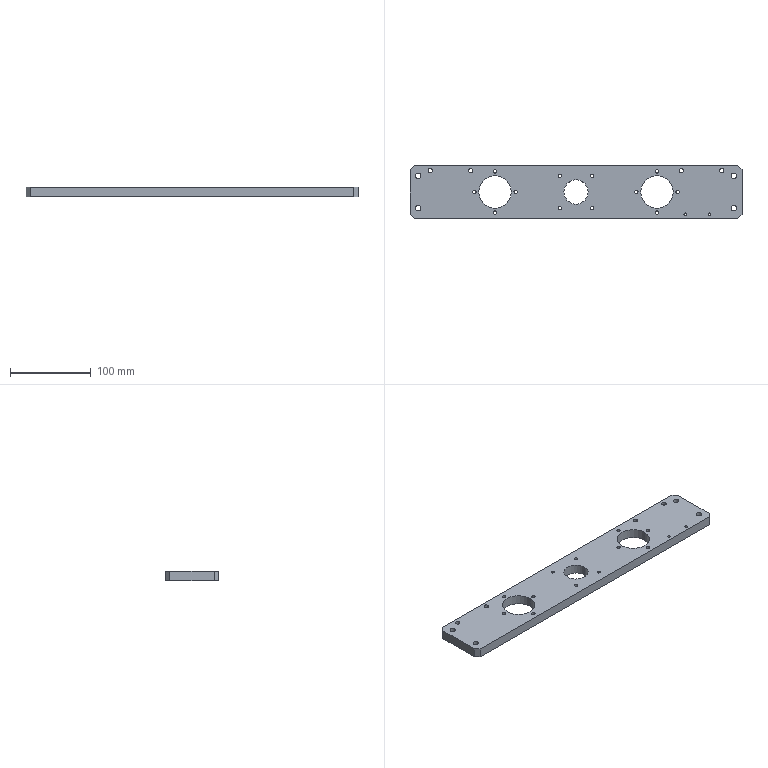Part | SolidWorks | features BaseBody 1 | 1 solid | 60 faces | box 410 x 65 x 12 mm | volume 275474 mm3 | cylinder 50 | plane 10 | commonest cylinder face diameters 4.2 x24 5.5 x8 6.8 x8 3.3 x4 40 x4 30 x2